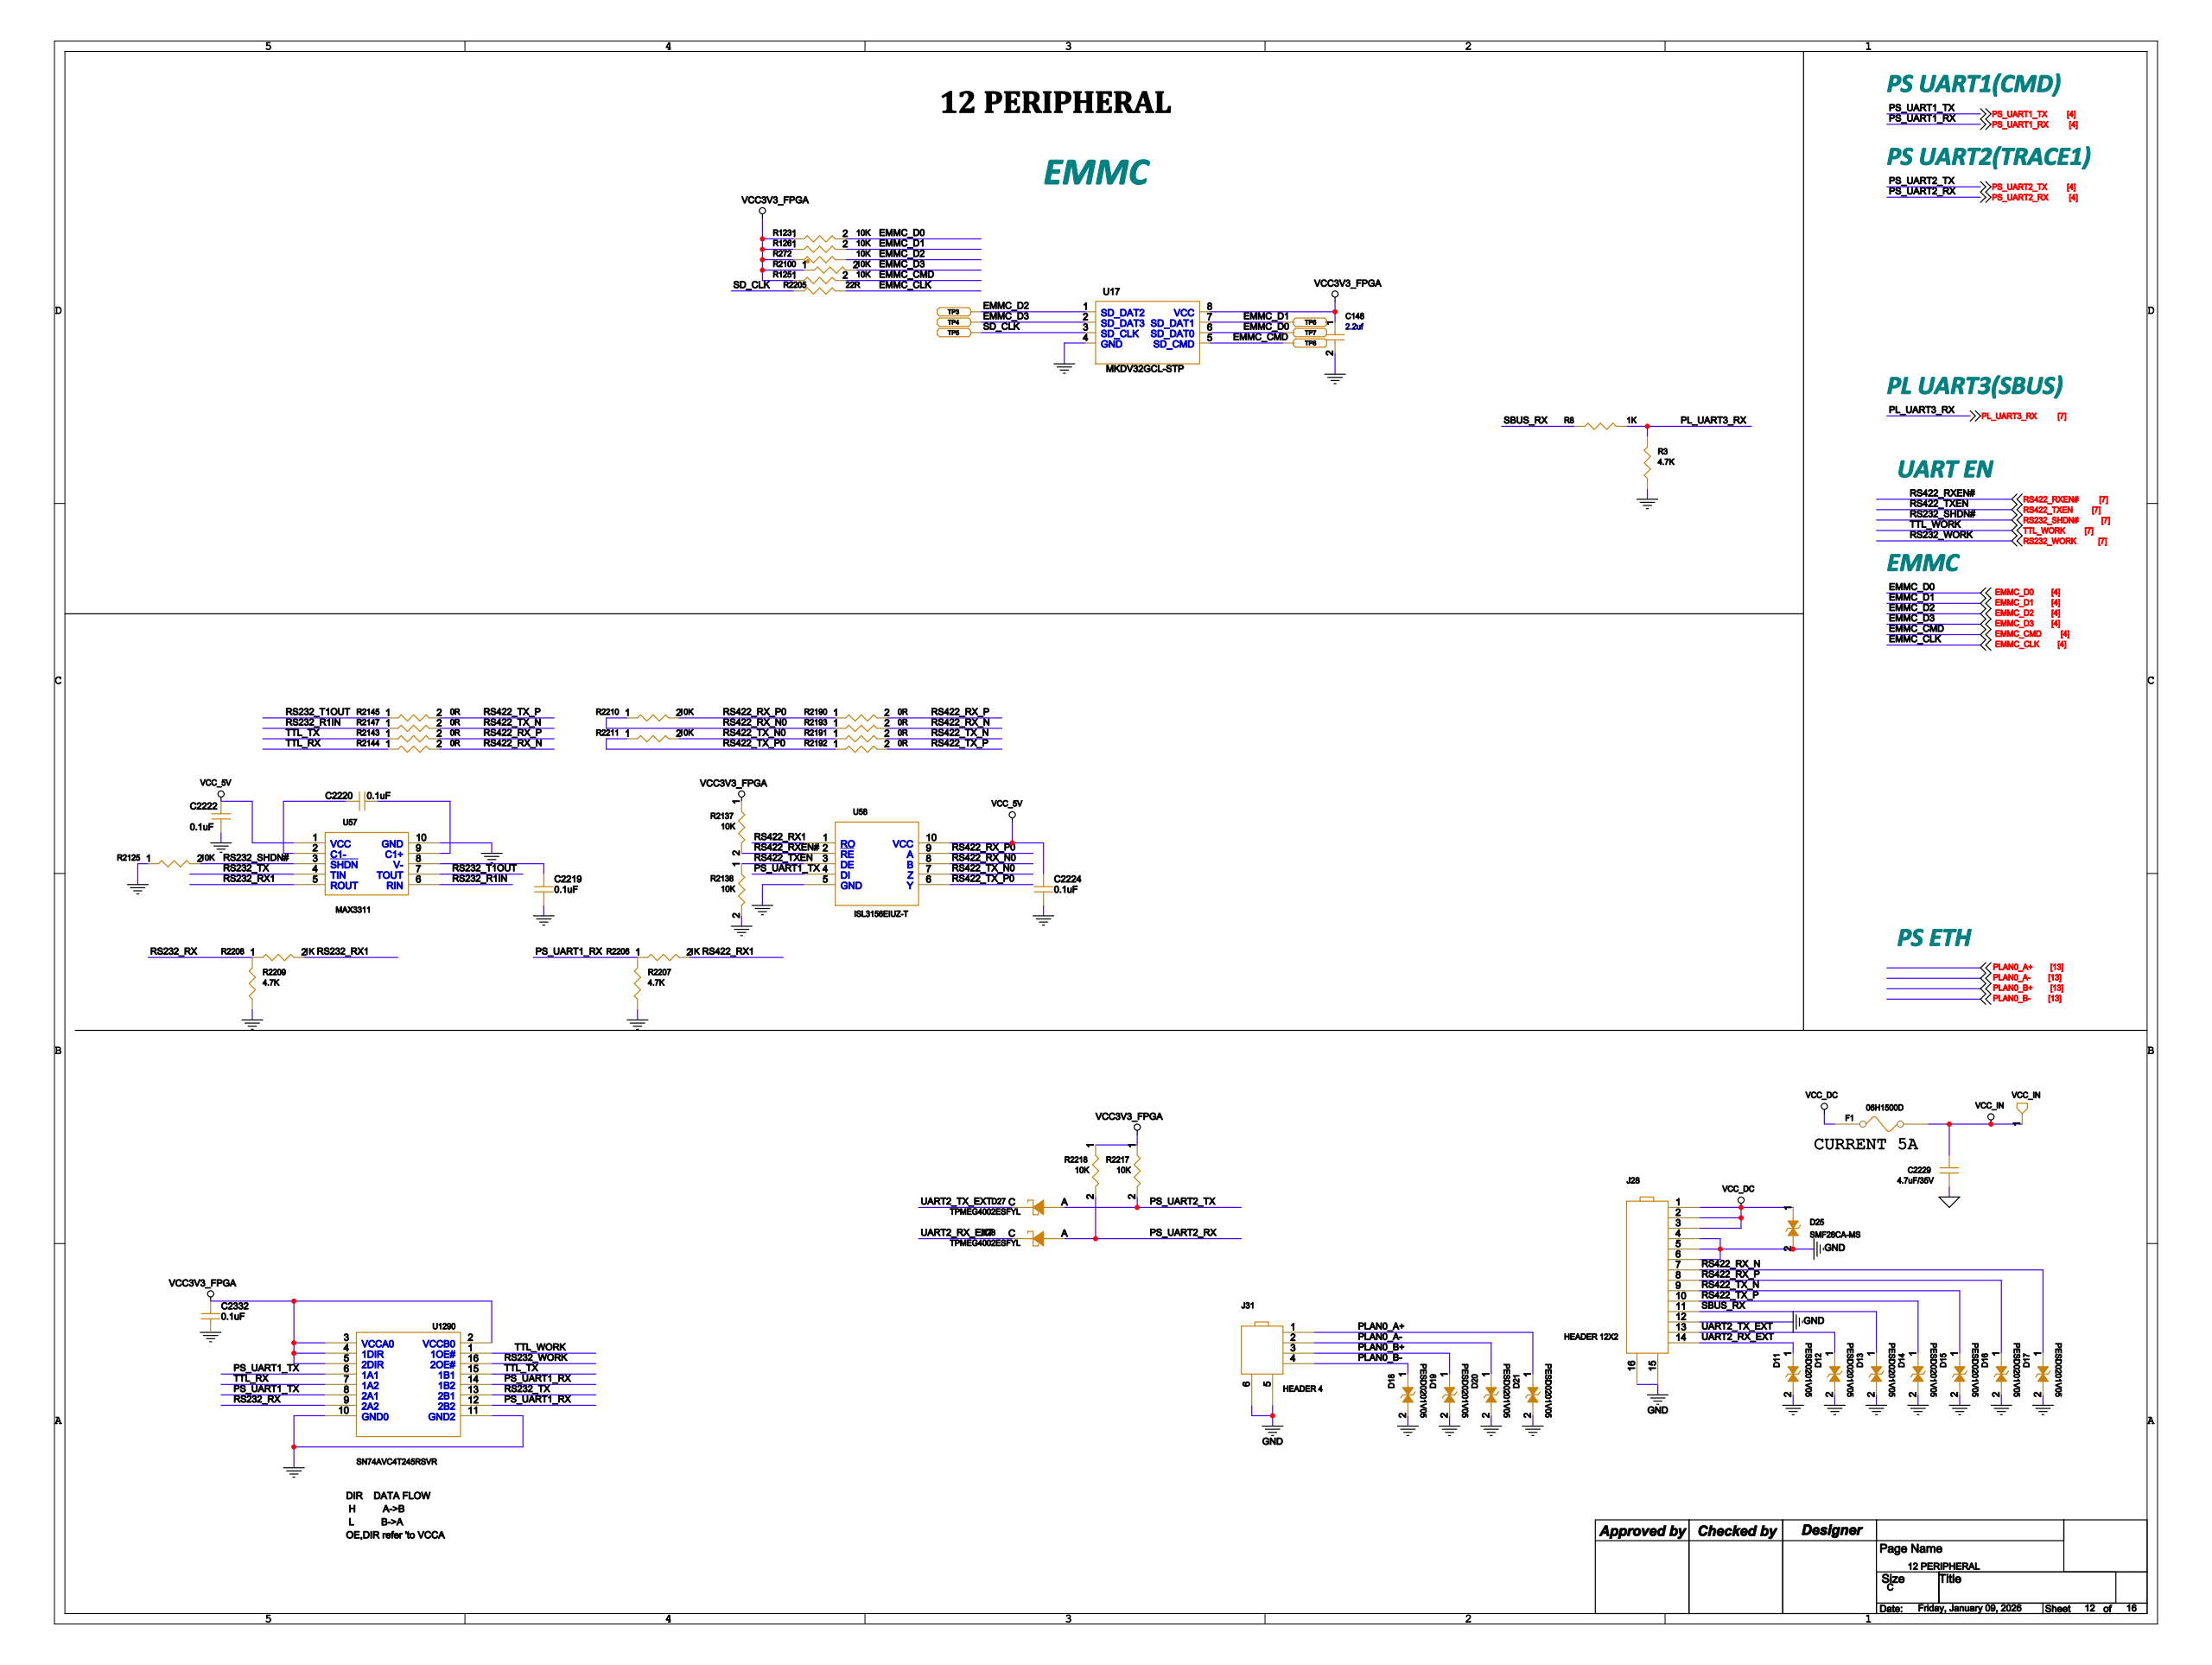Circuit board | Cadence Allegro | 442 parts | 326 nets | one sheet of the schematic
Parts on this sheet (reference | value | footprint):
C148 | 2.2uf | C0201
C2219 | 0.1uF | C0201
C2220 | 0.1uF | C0201
C2222 | 0.1uF | C0201
C2224 | 0.1uF | C0201
C2229 | 4.7uF/35V | C0603
C2332 | 0.1uF | C0201
D11 | PESD0201V05 | TVS0201
D12 | PESD0201V05 | TVS0201
D13 | PESD0201V05 | TVS0201
D14 | PESD0201V05 | TVS0201
D15 | PESD0201V05 | TVS0201
D16 | PESD0201V05 | TVS0201
D17 | PESD0201V05 | TVS0201
D18 | PESD0201V05 | TVS0201
D19 | PESD0201V05 | TVS0201
D20 | PESD0201V05 | TVS0201
D21 | PESD0201V05 | TVS0201
D25 | SMF28CA-MS | SOD-123FL
D27 | TPMEG4002ESFYL | D0201
D28 | TPMEG4002ESFYL | D0201
F1 | 06H1500D | R0603
J28 | HEADER 12X2 | 1MM25_14PIN
J31 | HEADER 4 | H-1MM25_4PIN
R3 | 4.7K | R0201
R8 | 1K | R0201
R272 | 10K | R0201
R2100 | 10K | R0201
R2125 | 10K | R0201
R2137 | 10K | R0201
R2138 | 10K | R0201
R2143 | 0R | R0201
R2144 | 0R | R0201
R2145 | 0R | R0201
R2147 | 0R | R0201
R2190 | 0R | R0201
R2191 | 0R | R0201
R2192 | 0R | R0201
R2193 | 0R | R0201
R2205 | 22R | R0201
R2206 | 1K | R0201
R2207 | 4.7K | R0201
R2208 | 1K | R0201
R2209 | 4.7K | R0201
R2210 | 10K | R0201
R2211 | 10K | R0201
R2217 | 10K | R0201
R2218 | 10K | R0201
TP3 | LABTESTPOINT | LTPT28C49P
TP4 | LABTESTPOINT | LTPT28C49P
TP5 | LABTESTPOINT | LTPT28C49P
TP6 | LABTESTPOINT | LTPT28C49P
TP7 | LABTESTPOINT | LTPT28C49P
TP8 | LABTESTPOINT | LTPT28C49P
U17 | MKDV32GCL-STP | MKDV32GCL-STP
U57 | MAX3311 | MSOP-10_1
U58 | ISL3156EIUZ-T | MSOP-10_1
U1290 | SN74AVC4T245RSVR | UQFN-16
Nets of these parts (net: part-pin ...):
VCC_5V: C2222-1 C2224-1 U57-1 U58-10
GND: C148-2 C2219-2 C2222-2 C2224-2 C2229-2 C2332-2 D11-2 D12-2 D13-2 D14-2 D15-2 D16-2 D17-2 D18-2 D19-2 D20-2 D21-2 D25-2 J28-4 J28-5 J28-6 J28-12 J28-15 J28-16 J31-5 J31-6 R3-2 R2125-1 R2138-2 R2207-2 R2209-2 U17-4 U57-10 U58-5 U1290-10 U1290-11
VCC_IN: C2229-1 F1-2
VCC_DC: D25-1 F1-1 J28-1 J28-2 J28-3
RS422_TX_P: D14-1 J28-10 R2145-2 R2192-2
SBUS_RX: D13-1 J28-11 R8-2
UART2_TX_EXT: D12-1 D27-C J28-13
UART2_RX_EXT: D11-1 D28-C J28-14
RS422_RX_N: D17-1 J28-7 R2144-2 R2193-2
RS422_RX_P: D16-1 J28-8 R2143-2 R2190-2
RS422_TX_N: D15-1 J28-9 R2147-2 R2191-2
PS_UART2_TX: D27-A R2217-2
PS_UART2_RX: D28-A R2218-2
PLAN0_B-: D18-1 J31-4
PLAN0_B+: D19-1 J31-3
PLAN0_A-: D20-1 J31-2
PLAN0_A+: D21-1 J31-1
PS_UART1_TX: U58-4 U1290-6 U1290-8
TTL_RX: R2144-1 U1290-7
TTL_TX: R2143-1 U1290-15
PS_UART1_RX: R2206-1 R2207-1 U1290-12 U1290-14
VCC3V3_FPGA: C148-1 C2332-1 R272-1 R2100-1 R2137-1 R2217-1 R2218-1 U17-8 U1290-2 U1290-3 U1290-4 U1290-5
TTL_WORK: U1290-1
RS232_RX: R2208-1 R2209-1 U1290-9
RS232_TX: U57-4 U1290-13
RS232_WORK: U1290-16
SD_CLK: R2205-2 TP5-1 U17-3
EMMC_CMD: TP8-1 U17-5
EMMC_D0: TP7-1 U17-6
EMMC_D1: TP6-1 U17-7
EMMC_D2: R272-2 TP3-1 U17-1
EMMC_D3: R2100-2 TP4-1 U17-2
RS422_RX_P0: R2190-1 R2210-2 U58-9
RS422_RX_N0: R2193-1 R2210-1 U58-8
RS422_TXEN: R2138-1 U58-3
RS422_RX1: R2206-2 U58-1
RS422_RXEN#: R2137-2 U58-2
RS422_TX_P0: R2192-1 R2211-1 U58-6
RS422_TX_N0: R2191-1 R2211-2 U58-7
EMMC_CLK: R2205-1
N50343853: C2220-1 U57-9
N50343368: C2220-2 U57-2
RS232_R1IN: R2147-1 U57-6
RS232_RX1: R2208-2 U57-5
RS232_SHDN#: R2125-2 U57-3
RS232_T1OUT: R2145-1 U57-7
N49929416: C2219-1 U57-8
PL_UART3_RX: R3-1 R8-1